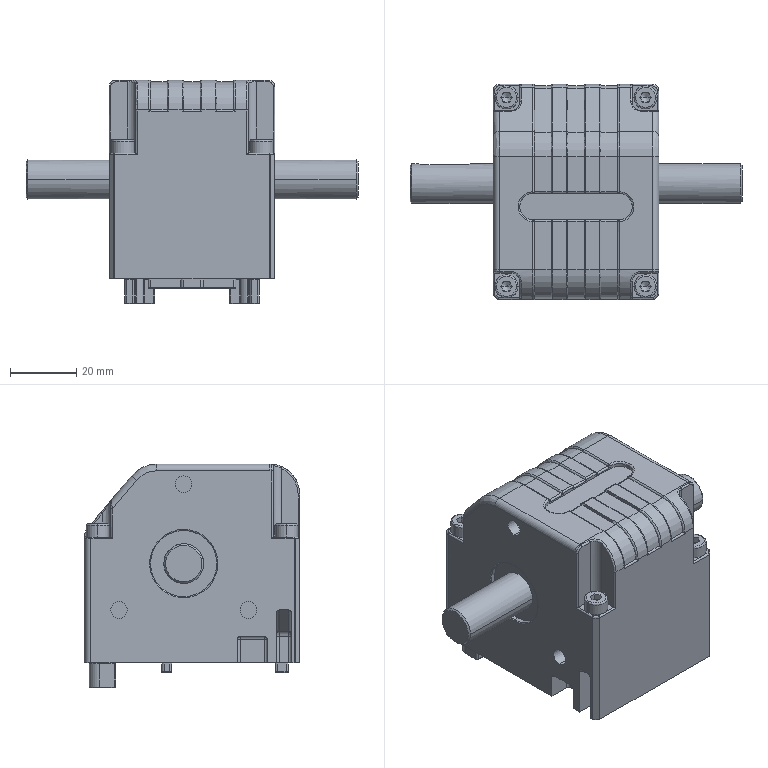Part | STEP file | Copy of K50-double output shaft^K50A-1H20-S(formula driven)-L300-motor left- | 7 solids | 723 faces | box 100.2 x 65 x 67.5 mm | volume 178596 mm3 | cylinder 297 | plane 210 | spline 188 | cone 28 | commonest cylinder face diameters 1 x85 5 x38 0.4 x24 4 x22 1.6 x18 0.6 x12